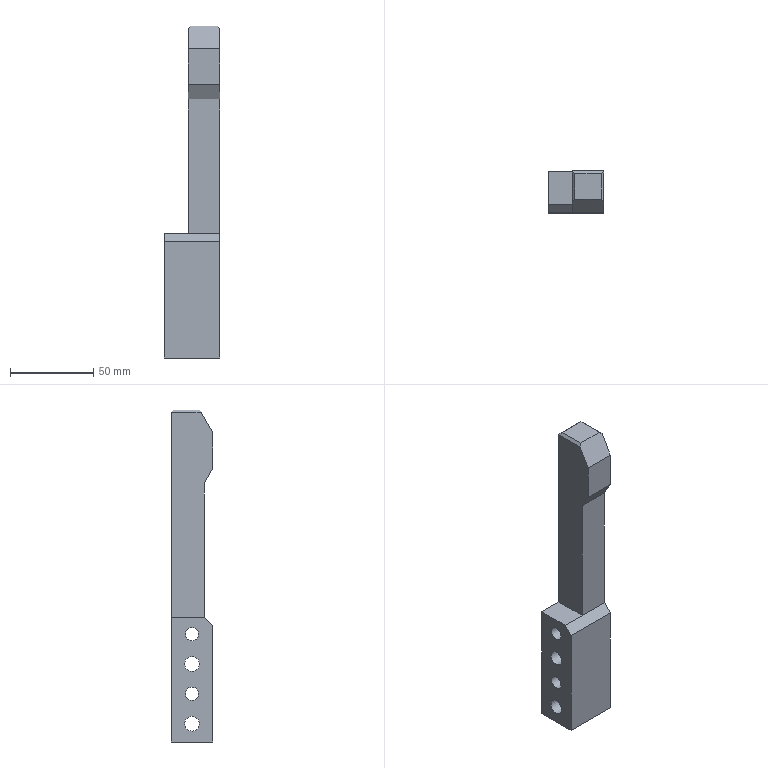Part | STEP file | solid 96 | 1 solid | 24 faces | box 33.5 x 25 x 199.996 mm | volume 103324 mm3 | plane 18 | cylinder 6 | commonest cylinder face diameters 8 x2 9 x2 14 x2